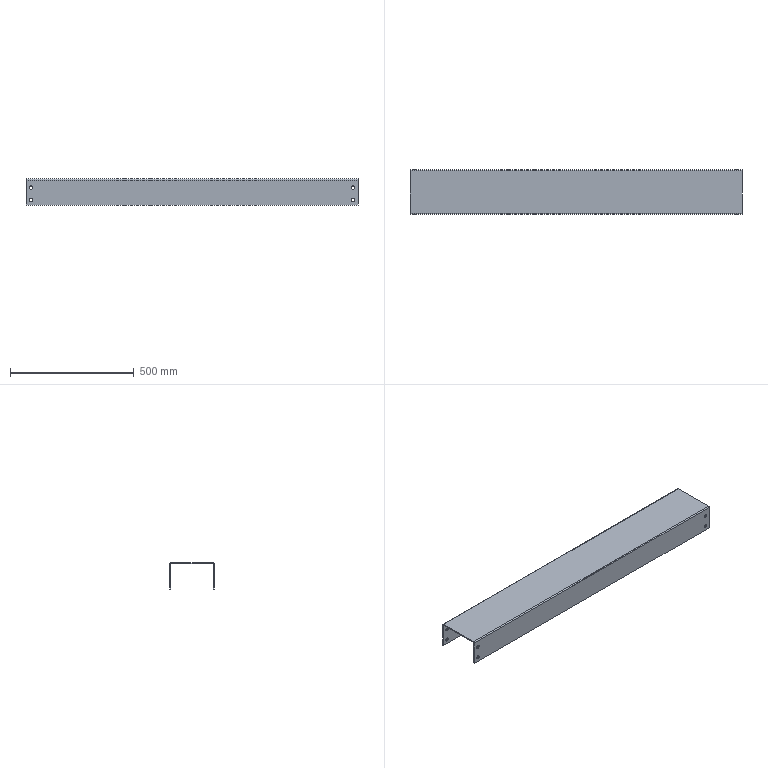Part | 1 solid | 38 faces | box 1340 x 180 x 105 mm | volume 2032472 mm3 | cylinder 20 | plane 18 | commonest cylinder face diameters 14 x16 0.4 x2 8.4 x2
STEP:
#1=CARTESIAN_POINT('',(650.,-90.,-92.));
#2=VERTEX_POINT('',#1);
#3=CARTESIAN_POINT('',(650.,-90.,-78.));
#4=VERTEX_POINT('',#3);
#5=CARTESIAN_POINT('',(650.,-90.,-85.));
#6=DIRECTION('',(0.,1.,0.));
#7=DIRECTION('',(0.,0.,1.));
#8=AXIS2_PLACEMENT_3D('',#5,#6,#7);
#9=CIRCLE('',#8,7.);
#10=EDGE_CURVE('',#2,#4,#9,.T.);
#11=ORIENTED_EDGE('',*,*,#10,.F.);
#12=CARTESIAN_POINT('',(650.,-86.,-92.));
#13=VERTEX_POINT('',#12);
#14=CARTESIAN_POINT('',(650.,-324.,-92.));
#15=DIRECTION('',(0.,1.,0.));
#16=VECTOR('',#15,1000.);
#17=LINE('',#14,#16);
#18=EDGE_CURVE('',#2,#13,#17,.T.);
#19=ORIENTED_EDGE('',*,*,#18,.T.);
#20=CARTESIAN_POINT('',(650.,-86.,-78.));
#21=VERTEX_POINT('',#20);
#22=CARTESIAN_POINT('',(650.,-86.,-85.));
#23=DIRECTION('',(0.,1.,0.));
#24=DIRECTION('',(0.,0.,1.));
#25=AXIS2_PLACEMENT_3D('',#22,#23,#24);
#26=CIRCLE('',#25,7.);
#27=EDGE_CURVE('',#13,#21,#26,.T.);
#28=ORIENTED_EDGE('',*,*,#27,.T.);
#29=CARTESIAN_POINT('',(650.,-324.,-78.));
#30=DIRECTION('',(0.,1.,0.));
#31=VECTOR('',#30,1000.);
#32=LINE('',#29,#31);
#33=EDGE_CURVE('',#4,#21,#32,.T.);
#34=ORIENTED_EDGE('',*,*,#33,.F.);
#35=EDGE_LOOP('',(#11,#19,#28,#34));
#36=FACE_OUTER_BOUND('',#35,.T.);
#37=CARTESIAN_POINT('',(650.,-324.,-85.));
#38=DIRECTION('',(0.,1.,0.));
#39=DIRECTION('',(0.,0.,1.));
#40=AXIS2_PLACEMENT_3D('',#37,#38,#39);
#41=CYLINDRICAL_SURFACE('',#40,7.);
#42=ADVANCED_FACE('',(#36),#41,.F.);
#43=CARTESIAN_POINT('',(650.,-90.,-42.));
#44=VERTEX_POINT('',#43);
#45=CARTESIAN_POINT('',(650.,-90.,-28.));
#46=VERTEX_POINT('',#45);
#47=CARTESIAN_POINT('',(650.,-90.,-35.));
#48=DIRECTION('',(0.,1.,0.));
#49=DIRECTION('',(0.,0.,1.));
#50=AXIS2_PLACEMENT_3D('',#47,#48,#49);
#51=CIRCLE('',#50,7.);
#52=EDGE_CURVE('',#44,#46,#51,.T.);
#53=ORIENTED_EDGE('',*,*,#52,.F.);
#54=CARTESIAN_POINT('',(650.,-86.,-42.));
#55=VERTEX_POINT('',#54);
#56=CARTESIAN_POINT('',(650.,-324.,-42.));
#57=DIRECTION('',(0.,1.,0.));
#58=VECTOR('',#57,1000.);
#59=LINE('',#56,#58);
#60=EDGE_CURVE('',#44,#55,#59,.T.);
#61=ORIENTED_EDGE('',*,*,#60,.T.);
#62=CARTESIAN_POINT('',(650.,-86.,-28.));
#63=VERTEX_POINT('',#62);
#64=CARTESIAN_POINT('',(650.,-86.,-35.));
#65=DIRECTION('',(0.,1.,0.));
#66=DIRECTION('',(0.,0.,1.));
#67=AXIS2_PLACEMENT_3D('',#64,#65,#66);
#68=CIRCLE('',#67,7.);
#69=EDGE_CURVE('',#55,#63,#68,.T.);
#70=ORIENTED_EDGE('',*,*,#69,.T.);
#71=CARTESIAN_POINT('',(650.,-324.,-28.));
#72=DIRECTION('',(0.,1.,0.));
#73=VECTOR('',#72,1000.);
#74=LINE('',#71,#73);
#75=EDGE_CURVE('',#46,#63,#74,.T.);
#76=ORIENTED_EDGE('',*,*,#75,.F.);
#77=EDGE_LOOP('',(#53,#61,#70,#76));
#78=FACE_OUTER_BOUND('',#77,.T.);
#79=CARTESIAN_POINT('',(650.,-324.,-35.));
#80=DIRECTION('',(0.,1.,0.));
#81=DIRECTION('',(0.,0.,1.));
#82=AXIS2_PLACEMENT_3D('',#79,#80,#81);
#83=CYLINDRICAL_SURFACE('',#82,7.);
#84=ADVANCED_FACE('',(#78),#83,.F.);
#85=CARTESIAN_POINT('',(-650.,-90.,-42.));
#86=VERTEX_POINT('',#85);
#87=CARTESIAN_POINT('',(-650.,-90.,-28.));
#88=VERTEX_POINT('',#87);
#89=CARTESIAN_POINT('',(-650.,-90.,-35.));
#90=DIRECTION('',(0.,1.,0.));
#91=DIRECTION('',(0.,0.,1.));
#92=AXIS2_PLACEMENT_3D('',#89,#90,#91);
#93=CIRCLE('',#92,7.);
#94=EDGE_CURVE('',#86,#88,#93,.T.);
#95=ORIENTED_EDGE('',*,*,#94,.F.);
#96=CARTESIAN_POINT('',(-650.,-86.,-42.));
#97=VERTEX_POINT('',#96);
#98=CARTESIAN_POINT('',(-650.,-324.,-42.));
#99=DIRECTION('',(0.,1.,0.));
#100=VECTOR('',#99,1000.);
#101=LINE('',#98,#100);
#102=EDGE_CURVE('',#86,#97,#101,.T.);
#103=ORIENTED_EDGE('',*,*,#102,.T.);
#104=CARTESIAN_POINT('',(-650.,-86.,-28.));
#105=VERTEX_POINT('',#104);
#106=CARTESIAN_POINT('',(-650.,-86.,-35.));
#107=DIRECTION('',(0.,1.,0.));
#108=DIRECTION('',(0.,0.,1.));
#109=AXIS2_PLACEMENT_3D('',#106,#107,#108);
#110=CIRCLE('',#109,7.);
#111=EDGE_CURVE('',#97,#105,#110,.T.);
#112=ORIENTED_EDGE('',*,*,#111,.T.);
#113=CARTESIAN_POINT('',(-650.,-324.,-28.));
#114=DIRECTION('',(0.,1.,0.));
#115=VECTOR('',#114,1000.);
#116=LINE('',#113,#115);
#117=EDGE_CURVE('',#88,#105,#116,.T.);
#118=ORIENTED_EDGE('',*,*,#117,.F.);
#119=EDGE_LOOP('',(#95,#103,#112,#118));
#120=FACE_OUTER_BOUND('',#119,.T.);
#121=CARTESIAN_POINT('',(-650.,-324.,-35.));
#122=DIRECTION('',(0.,1.,0.));
#123=DIRECTION('',(0.,0.,1.));
#124=AXIS2_PLACEMENT_3D('',#121,#122,#123);
#125=CYLINDRICAL_SURFACE('',#124,7.);
#126=ADVANCED_FACE('',(#120),#125,.F.);
#127=CARTESIAN_POINT('',(-650.,-90.,-92.));
#128=VERTEX_POINT('',#127);
#129=CARTESIAN_POINT('',(-650.,-90.,-78.));
#130=VERTEX_POINT('',#129);
#131=CARTESIAN_POINT('',(-650.,-90.,-85.));
#132=DIRECTION('',(0.,1.,0.));
#133=DIRECTION('',(0.,0.,1.));
#134=AXIS2_PLACEMENT_3D('',#131,#132,#133);
#135=CIRCLE('',#134,7.);
#136=EDGE_CURVE('',#128,#130,#135,.T.);
#137=ORIENTED_EDGE('',*,*,#136,.F.);
#138=CARTESIAN_POINT('',(-650.,-86.,-92.));
#139=VERTEX_POINT('',#138);
#140=CARTESIAN_POINT('',(-650.,-324.,-92.));
#141=DIRECTION('',(0.,1.,0.));
#142=VECTOR('',#141,1000.);
#143=LINE('',#140,#142);
#144=EDGE_CURVE('',#128,#139,#143,.T.);
#145=ORIENTED_EDGE('',*,*,#144,.T.);
#146=CARTESIAN_POINT('',(-650.,-86.,-78.));
#147=VERTEX_POINT('',#146);
#148=CARTESIAN_POINT('',(-650.,-86.,-85.));
#149=DIRECTION('',(0.,1.,0.));
#150=DIRECTION('',(0.,0.,1.));
#151=AXIS2_PLACEMENT_3D('',#148,#149,#150);
#152=CIRCLE('',#151,7.);
#153=EDGE_CURVE('',#139,#147,#152,.T.);
#154=ORIENTED_EDGE('',*,*,#153,.T.);
#155=CARTESIAN_POINT('',(-650.,-324.,-78.));
#156=DIRECTION('',(0.,1.,0.));
#157=VECTOR('',#156,1000.);
#158=LINE('',#155,#157);
#159=EDGE_CURVE('',#130,#147,#158,.T.);
#160=ORIENTED_EDGE('',*,*,#159,.F.);
#161=EDGE_LOOP('',(#137,#145,#154,#160));
#162=FACE_OUTER_BOUND('',#161,.T.);
#163=CARTESIAN_POINT('',(-650.,-324.,-85.));
#164=DIRECTION('',(0.,1.,0.));
#165=DIRECTION('',(0.,0.,1.));
#166=AXIS2_PLACEMENT_3D('',#163,#164,#165);
#167=CYLINDRICAL_SURFACE('',#166,7.);
#168=ADVANCED_FACE('',(#162),#167,.F.);
#169=CARTESIAN_POINT('',(650.,86.,-78.));
#170=VERTEX_POINT('',#169);
#171=CARTESIAN_POINT('',(650.,86.,-92.));
#172=VERTEX_POINT('',#171);
#173=CARTESIAN_POINT('',(650.,86.,-85.));
#174=DIRECTION('',(0.,-1.,0.));
#175=DIRECTION('',(0.,0.,-1.));
#176=AXIS2_PLACEMENT_3D('',#173,#174,#175);
#177=CIRCLE('',#176,7.);
#178=EDGE_CURVE('',#170,#172,#177,.T.);
#179=ORIENTED_EDGE('',*,*,#178,.T.);
#180=CARTESIAN_POINT('',(650.,90.,-92.));
#181=VERTEX_POINT('',#180);
#182=CARTESIAN_POINT('',(650.,-324.,-92.));
#183=DIRECTION('',(0.,1.,0.));
#184=VECTOR('',#183,1000.);
#185=LINE('',#182,#184);
#186=EDGE_CURVE('',#172,#181,#185,.T.);
#187=ORIENTED_EDGE('',*,*,#186,.T.);
#188=CARTESIAN_POINT('',(650.,90.,-78.));
#189=VERTEX_POINT('',#188);
#190=CARTESIAN_POINT('',(650.,90.,-85.));
#191=DIRECTION('',(0.,1.,0.));
#192=DIRECTION('',(0.,0.,-1.));
#193=AXIS2_PLACEMENT_3D('',#190,#191,#192);
#194=CIRCLE('',#193,7.);
#195=EDGE_CURVE('',#181,#189,#194,.T.);
#196=ORIENTED_EDGE('',*,*,#195,.T.);
#197=CARTESIAN_POINT('',(650.,-324.,-78.));
#198=DIRECTION('',(0.,1.,0.));
#199=VECTOR('',#198,1000.);
#200=LINE('',#197,#199);
#201=EDGE_CURVE('',#170,#189,#200,.T.);
#202=ORIENTED_EDGE('',*,*,#201,.F.);
#203=EDGE_LOOP('',(#179,#187,#196,#202));
#204=FACE_OUTER_BOUND('',#203,.T.);
#205=CARTESIAN_POINT('',(650.,-324.,-85.));
#206=DIRECTION('',(0.,1.,0.));
#207=DIRECTION('',(0.,0.,1.));
#208=AXIS2_PLACEMENT_3D('',#205,#206,#207);
#209=CYLINDRICAL_SURFACE('',#208,7.);
#210=ADVANCED_FACE('',(#204),#209,.F.);
#211=CARTESIAN_POINT('',(650.,86.,-28.));
#212=VERTEX_POINT('',#211);
#213=CARTESIAN_POINT('',(650.,86.,-42.));
#214=VERTEX_POINT('',#213);
#215=CARTESIAN_POINT('',(650.,86.,-35.));
#216=DIRECTION('',(0.,-1.,0.));
#217=DIRECTION('',(0.,0.,-1.));
#218=AXIS2_PLACEMENT_3D('',#215,#216,#217);
#219=CIRCLE('',#218,7.);
#220=EDGE_CURVE('',#212,#214,#219,.T.);
#221=ORIENTED_EDGE('',*,*,#220,.T.);
#222=CARTESIAN_POINT('',(650.,90.,-42.));
#223=VERTEX_POINT('',#222);
#224=CARTESIAN_POINT('',(650.,-324.,-42.));
#225=DIRECTION('',(0.,1.,0.));
#226=VECTOR('',#225,1000.);
#227=LINE('',#224,#226);
#228=EDGE_CURVE('',#214,#223,#227,.T.);
#229=ORIENTED_EDGE('',*,*,#228,.T.);
#230=CARTESIAN_POINT('',(650.,90.,-28.));
#231=VERTEX_POINT('',#230);
#232=CARTESIAN_POINT('',(650.,90.,-35.));
#233=DIRECTION('',(0.,1.,0.));
#234=DIRECTION('',(0.,0.,-1.));
#235=AXIS2_PLACEMENT_3D('',#232,#233,#234);
#236=CIRCLE('',#235,7.);
#237=EDGE_CURVE('',#223,#231,#236,.T.);
#238=ORIENTED_EDGE('',*,*,#237,.T.);
#239=CARTESIAN_POINT('',(650.,-324.,-28.));
#240=DIRECTION('',(0.,1.,0.));
#241=VECTOR('',#240,1000.);
#242=LINE('',#239,#241);
#243=EDGE_CURVE('',#212,#231,#242,.T.);
#244=ORIENTED_EDGE('',*,*,#243,.F.);
#245=EDGE_LOOP('',(#221,#229,#238,#244));
#246=FACE_OUTER_BOUND('',#245,.T.);
#247=CARTESIAN_POINT('',(650.,-324.,-35.));
#248=DIRECTION('',(0.,1.,0.));
#249=DIRECTION('',(0.,0.,1.));
#250=AXIS2_PLACEMENT_3D('',#247,#248,#249);
#251=CYLINDRICAL_SURFACE('',#250,7.);
#252=ADVANCED_FACE('',(#246),#251,.F.);
#253=CARTESIAN_POINT('',(-650.,86.,-28.));
#254=VERTEX_POINT('',#253);
#255=CARTESIAN_POINT('',(-650.,86.,-42.));
#256=VERTEX_POINT('',#255);
#257=CARTESIAN_POINT('',(-650.,86.,-35.));
#258=DIRECTION('',(0.,-1.,0.));
#259=DIRECTION('',(0.,0.,-1.));
#260=AXIS2_PLACEMENT_3D('',#257,#258,#259);
#261=CIRCLE('',#260,7.);
#262=EDGE_CURVE('',#254,#256,#261,.T.);
#263=ORIENTED_EDGE('',*,*,#262,.T.);
#264=CARTESIAN_POINT('',(-650.,90.,-42.));
#265=VERTEX_POINT('',#264);
#266=CARTESIAN_POINT('',(-650.,-324.,-42.));
#267=DIRECTION('',(0.,1.,0.));
#268=VECTOR('',#267,1000.);
#269=LINE('',#266,#268);
#270=EDGE_CURVE('',#256,#265,#269,.T.);
#271=ORIENTED_EDGE('',*,*,#270,.T.);
#272=CARTESIAN_POINT('',(-650.,90.,-28.));
#273=VERTEX_POINT('',#272);
#274=CARTESIAN_POINT('',(-650.,90.,-35.));
#275=DIRECTION('',(0.,1.,0.));
#276=DIRECTION('',(0.,0.,1.));
#277=AXIS2_PLACEMENT_3D('',#274,#275,#276);
#278=CIRCLE('',#277,7.);
#279=EDGE_CURVE('',#265,#273,#278,.T.);
#280=ORIENTED_EDGE('',*,*,#279,.T.);
#281=CARTESIAN_POINT('',(-650.,-324.,-28.));
#282=DIRECTION('',(0.,1.,0.));
#283=VECTOR('',#282,1000.);
#284=LINE('',#281,#283);
#285=EDGE_CURVE('',#254,#273,#284,.T.);
#286=ORIENTED_EDGE('',*,*,#285,.F.);
#287=EDGE_LOOP('',(#263,#271,#280,#286));
#288=FACE_OUTER_BOUND('',#287,.T.);
#289=CARTESIAN_POINT('',(-650.,-324.,-35.));
#290=DIRECTION('',(0.,1.,0.));
#291=DIRECTION('',(0.,0.,1.));
#292=AXIS2_PLACEMENT_3D('',#289,#290,#291);
#293=CYLINDRICAL_SURFACE('',#292,7.);
#294=ADVANCED_FACE('',(#288),#293,.F.);
#295=CARTESIAN_POINT('',(-650.,86.,-78.));
#296=VERTEX_POINT('',#295);
#297=CARTESIAN_POINT('',(-650.,86.,-92.));
#298=VERTEX_POINT('',#297);
#299=CARTESIAN_POINT('',(-650.,86.,-85.));
#300=DIRECTION('',(0.,-1.,0.));
#301=DIRECTION('',(0.,0.,-1.));
#302=AXIS2_PLACEMENT_3D('',#299,#300,#301);
#303=CIRCLE('',#302,7.);
#304=EDGE_CURVE('',#296,#298,#303,.T.);
#305=ORIENTED_EDGE('',*,*,#304,.T.);
#306=CARTESIAN_POINT('',(-650.,90.,-92.));
#307=VERTEX_POINT('',#306);
#308=CARTESIAN_POINT('',(-650.,-324.,-92.));
#309=DIRECTION('',(0.,1.,0.));
#310=VECTOR('',#309,1000.);
#311=LINE('',#308,#310);
#312=EDGE_CURVE('',#298,#307,#311,.T.);
#313=ORIENTED_EDGE('',*,*,#312,.T.);
#314=CARTESIAN_POINT('',(-650.,90.,-78.));
#315=VERTEX_POINT('',#314);
#316=CARTESIAN_POINT('',(-650.,90.,-85.));
#317=DIRECTION('',(0.,1.,0.));
#318=DIRECTION('',(0.,0.,1.));
#319=AXIS2_PLACEMENT_3D('',#316,#317,#318);
#320=CIRCLE('',#319,7.);
#321=EDGE_CURVE('',#307,#315,#320,.T.);
#322=ORIENTED_EDGE('',*,*,#321,.T.);
#323=CARTESIAN_POINT('',(-650.,-324.,-78.));
#324=DIRECTION('',(0.,1.,0.));
#325=VECTOR('',#324,1000.);
#326=LINE('',#323,#325);
#327=EDGE_CURVE('',#296,#315,#326,.T.);
#328=ORIENTED_EDGE('',*,*,#327,.F.);
#329=EDGE_LOOP('',(#305,#313,#322,#328));
#330=FACE_OUTER_BOUND('',#329,.T.);
#331=CARTESIAN_POINT('',(-650.,-324.,-85.));
#332=DIRECTION('',(0.,1.,0.));
#333=DIRECTION('',(0.,0.,1.));
#334=AXIS2_PLACEMENT_3D('',#331,#332,#333);
#335=CYLINDRICAL_SURFACE('',#334,7.);
#336=ADVANCED_FACE('',(#330),#335,.F.);
#337=CARTESIAN_POINT('',(670.,90.,-4.2));
#338=VERTEX_POINT('',#337);
#339=CARTESIAN_POINT('',(670.,86.,-4.2));
#340=VERTEX_POINT('',#339);
#341=CARTESIAN_POINT('',(670.,90.,-4.2));
#342=DIRECTION('',(0.,-1.,0.));
#343=VECTOR('',#342,1000.);
#344=LINE('',#341,#343);
#345=EDGE_CURVE('',#338,#340,#344,.T.);
#346=ORIENTED_EDGE('',*,*,#345,.F.);
#347=CARTESIAN_POINT('',(670.,85.8,0.));
#348=VERTEX_POINT('',#347);
#349=CARTESIAN_POINT('',(670.,85.8,-4.2));
#350=DIRECTION('',(1.,0.,0.));
#351=DIRECTION('',(0.,0.,1.));
#352=AXIS2_PLACEMENT_3D('',#349,#350,#351);
#353=CIRCLE('',#352,4.2);
#354=EDGE_CURVE('',#338,#348,#353,.T.);
#355=ORIENTED_EDGE('',*,*,#354,.T.);
#356=CARTESIAN_POINT('',(670.,85.8,-4.));
#357=VERTEX_POINT('',#356);
#358=CARTESIAN_POINT('',(670.,85.8,-4.));
#359=DIRECTION('',(0.,0.,1.));
#360=VECTOR('',#359,1000.);
#361=LINE('',#358,#360);
#362=EDGE_CURVE('',#357,#348,#361,.T.);
#363=ORIENTED_EDGE('',*,*,#362,.F.);
#364=CARTESIAN_POINT('',(670.,85.8,-4.2));
#365=DIRECTION('',(1.,0.,0.));
#366=DIRECTION('',(0.,0.,-1.));
#367=AXIS2_PLACEMENT_3D('',#364,#365,#366);
#368=CIRCLE('',#367,0.2);
#369=EDGE_CURVE('',#340,#357,#368,.T.);
#370=ORIENTED_EDGE('',*,*,#369,.F.);
#371=EDGE_LOOP('',(#346,#355,#363,#370));
#372=FACE_OUTER_BOUND('',#371,.T.);
#373=CARTESIAN_POINT('',(670.,90.,-4.2));
#374=DIRECTION('',(1.,0.,0.));
#375=DIRECTION('',(0.,0.,-1.));
#376=AXIS2_PLACEMENT_3D('',#373,#374,#375);
#377=PLANE('',#376);
#378=ADVANCED_FACE('',(#372),#377,.T.);
#379=CARTESIAN_POINT('',(670.,90.,-105.));
#380=VERTEX_POINT('',#379);
#381=CARTESIAN_POINT('',(670.,90.,-105.));
#382=DIRECTION('',(0.,0.,1.));
#383=VECTOR('',#382,1000.);
#384=LINE('',#381,#383);
#385=EDGE_CURVE('',#380,#338,#384,.T.);
#386=ORIENTED_EDGE('',*,*,#385,.T.);
#387=ORIENTED_EDGE('',*,*,#345,.T.);
#388=CARTESIAN_POINT('',(670.,86.,-105.));
#389=VERTEX_POINT('',#388);
#390=CARTESIAN_POINT('',(670.,86.,-105.));
#391=DIRECTION('',(0.,0.,1.));
#392=VECTOR('',#391,1000.);
#393=LINE('',#390,#392);
#394=EDGE_CURVE('',#389,#340,#393,.T.);
#395=ORIENTED_EDGE('',*,*,#394,.F.);
#396=CARTESIAN_POINT('',(670.,90.,-105.));
#397=DIRECTION('',(0.,-1.,0.));
#398=VECTOR('',#397,1000.);
#399=LINE('',#396,#398);
#400=EDGE_CURVE('',#380,#389,#399,.T.);
#401=ORIENTED_EDGE('',*,*,#400,.F.);
#402=EDGE_LOOP('',(#386,#387,#395,#401));
#403=FACE_OUTER_BOUND('',#402,.T.);
#404=CARTESIAN_POINT('',(670.,85.8,-4.));
#405=DIRECTION('',(1.,0.,0.));
#406=DIRECTION('',(0.,0.,-1.));
#407=AXIS2_PLACEMENT_3D('',#404,#405,#406);
#408=PLANE('',#407);
#409=ADVANCED_FACE('',(#403),#408,.T.);
#410=CARTESIAN_POINT('',(-670.,85.8,0.));
#411=VERTEX_POINT('',#410);
#412=CARTESIAN_POINT('',(-670.,85.8,-4.));
#413=VERTEX_POINT('',#412);
#414=CARTESIAN_POINT('',(-670.,85.8,0.));
#415=DIRECTION('',(0.,0.,-1.));
#416=VECTOR('',#415,1000.);
#417=LINE('',#414,#416);
#418=EDGE_CURVE('',#411,#413,#417,.T.);
#419=ORIENTED_EDGE('',*,*,#418,.F.);
#420=CARTESIAN_POINT('',(-670.,90.,-4.2));
#421=VERTEX_POINT('',#420);
#422=CARTESIAN_POINT('',(-670.,85.8,-4.2));
#423=DIRECTION('',(1.,0.,0.));
#424=DIRECTION('',(0.,0.,1.));
#425=AXIS2_PLACEMENT_3D('',#422,#423,#424);
#426=CIRCLE('',#425,4.2);
#427=EDGE_CURVE('',#421,#411,#426,.T.);
#428=ORIENTED_EDGE('',*,*,#427,.F.);
#429=CARTESIAN_POINT('',(-670.,86.,-4.2));
#430=VERTEX_POINT('',#429);
#431=CARTESIAN_POINT('',(-670.,86.,-4.2));
#432=DIRECTION('',(0.,1.,0.));
#433=VECTOR('',#432,1000.);
#434=LINE('',#431,#433);
#435=EDGE_CURVE('',#430,#421,#434,.T.);
#436=ORIENTED_EDGE('',*,*,#435,.F.);
#437=CARTESIAN_POINT('',(-670.,85.8,-4.2));
#438=DIRECTION('',(1.,0.,0.));
#439=DIRECTION('',(0.,0.,-1.));
#440=AXIS2_PLACEMENT_3D('',#437,#438,#439);
#441=CIRCLE('',#440,0.2);
#442=EDGE_CURVE('',#430,#413,#441,.T.);
#443=ORIENTED_EDGE('',*,*,#442,.T.);
#444=EDGE_LOOP('',(#419,#428,#436,#443));
#445=FACE_OUTER_BOUND('',#444,.T.);
#446=CARTESIAN_POINT('',(-670.,85.8,0.));
#447=DIRECTION('',(-1.,0.,0.));
#448=DIRECTION('',(0.,0.,1.));
#449=AXIS2_PLACEMENT_3D('',#446,#447,#448);
#450=PLANE('',#449);
#451=ADVANCED_FACE('',(#445),#450,.T.);
#452=CARTESIAN_POINT('',(-670.,-85.8,0.));
#453=VERTEX_POINT('',#452);
#454=CARTESIAN_POINT('',(-670.,90.,0.));
#455=DIRECTION('',(0.,-1.,0.));
#456=VECTOR('',#455,1000.);
#457=LINE('',#454,#456);
#458=EDGE_CURVE('',#411,#453,#457,.T.);
#459=ORIENTED_EDGE('',*,*,#458,.F.);
#460=ORIENTED_EDGE('',*,*,#418,.T.);
#461=CARTESIAN_POINT('',(-670.,-85.8,-4.));
#462=VERTEX_POINT('',#461);
#463=CARTESIAN_POINT('',(-670.,90.,-4.));
#464=DIRECTION('',(0.,-1.,0.));
#465=VECTOR('',#464,1000.);
#466=LINE('',#463,#465);
#467=EDGE_CURVE('',#413,#462,#466,.T.);
#468=ORIENTED_EDGE('',*,*,#467,.T.);
#469=CARTESIAN_POINT('',(-670.,-85.8,-4.));
#470=DIRECTION('',(0.,0.,1.));
#471=VECTOR('',#470,1000.);
#472=LINE('',#469,#471);
#473=EDGE_CURVE('',#462,#453,#472,.T.);
#474=ORIENTED_EDGE('',*,*,#473,.T.);
#475=EDGE_LOOP('',(#459,#460,#468,#474));
#476=FACE_OUTER_BOUND('',#475,.T.);
#477=CARTESIAN_POINT('',(-670.,86.,-4.2));
#478=DIRECTION('',(-1.,0.,0.));
#479=DIRECTION('',(0.,0.,1.));
#480=AXIS2_PLACEMENT_3D('',#477,#478,#479);
#481=PLANE('',#480);
#482=ADVANCED_FACE('',(#476),#481,.T.);
#483=CARTESIAN_POINT('',(670.,-85.8,0.));
#484=VERTEX_POINT('',#483);
#485=CARTESIAN_POINT('',(670.,-85.8,-4.));
#486=VERTEX_POINT('',#485);
#487=CARTESIAN_POINT('',(670.,-85.8,0.));
#488=DIRECTION('',(0.,0.,-1.));
#489=VECTOR('',#488,1000.);
#490=LINE('',#487,#489);
#491=EDGE_CURVE('',#484,#486,#490,.T.);
#492=ORIENTED_EDGE('',*,*,#491,.F.);
#493=CARTESIAN_POINT('',(670.,-90.,-4.2));
#494=VERTEX_POINT('',#493);
#495=CARTESIAN_POINT('',(670.,-85.8,-4.2));
#496=DIRECTION('',(1.,0.,0.));
#497=DIRECTION('',(0.,0.,1.));
#498=AXIS2_PLACEMENT_3D('',#495,#496,#497);
#499=CIRCLE('',#498,4.2);
#500=EDGE_CURVE('',#484,#494,#499,.T.);
#501=ORIENTED_EDGE('',*,*,#500,.T.);
#502=CARTESIAN_POINT('',(670.,-86.,-4.2));
#503=VERTEX_POINT('',#502);
#504=CARTESIAN_POINT('',(670.,-86.,-4.2));
#505=DIRECTION('',(0.,-1.,0.));
#506=VECTOR('',#505,1000.);
#507=LINE('',#504,#506);
#508=EDGE_CURVE('',#503,#494,#507,.T.);
#509=ORIENTED_EDGE('',*,*,#508,.F.);
#510=CARTESIAN_POINT('',(670.,-85.8,-4.2));
#511=DIRECTION('',(1.,0.,0.));
#512=DIRECTION('',(0.,0.,-1.));
#513=AXIS2_PLACEMENT_3D('',#510,#511,#512);
#514=CIRCLE('',#513,0.2);
#515=EDGE_CURVE('',#486,#503,#514,.T.);
#516=ORIENTED_EDGE('',*,*,#515,.F.);
#517=EDGE_LOOP('',(#492,#501,#509,#516));
#518=FACE_OUTER_BOUND('',#517,.T.);
#519=CARTESIAN_POINT('',(670.,-85.8,0.));
#520=DIRECTION('',(1.,0.,0.));
#521=DIRECTION('',(0.,0.,-1.));
#522=AXIS2_PLACEMENT_3D('',#519,#520,#521);
#523=PLANE('',#522);
#524=ADVANCED_FACE('',(#518),#523,.T.);
#525=CARTESIAN_POINT('',(670.,90.,0.));
#526=DIRECTION('',(0.,-1.,0.));
#527=VECTOR('',#526,1000.);
#528=LINE('',#525,#527);
#529=EDGE_CURVE('',#348,#484,#528,.T.);
#530=ORIENTED_EDGE('',*,*,#529,.T.);
#531=ORIENTED_EDGE('',*,*,#491,.T.);
#532=CARTESIAN_POINT('',(670.,90.,-4.));
#533=DIRECTION('',(0.,-1.,0.));
#534=VECTOR('',#533,1000.);
#535=LINE('',#532,#534);
#536=EDGE_CURVE('',#357,#486,#535,.T.);
#537=ORIENTED_EDGE('',*,*,#536,.F.);
#538=ORIENTED_EDGE('',*,*,#362,.T.);
#539=EDGE_LOOP('',(#530,#531,#537,#538));
#540=FACE_OUTER_BOUND('',#539,.T.);
#541=CARTESIAN_POINT('',(670.,-86.,-4.2));
#542=DIRECTION('',(1.,0.,0.));
#543=DIRECTION('',(0.,0.,-1.));
#544=AXIS2_PLACEMENT_3D('',#541,#542,#543);
#545=PLANE('',#544);
#546=ADVANCED_FACE('',(#540),#545,.T.);
#547=CARTESIAN_POINT('',(-670.,-90.,-4.2));
#548=VERTEX_POINT('',#547);
#549=CARTESIAN_POINT('',(-670.,-86.,-4.2));
#550=VERTEX_POINT('',#549);
#551=CARTESIAN_POINT('',(-670.,-90.,-4.2));
#552=DIRECTION('',(0.,1.,0.));
#553=VECTOR('',#552,1000.);
#554=LINE('',#551,#553);
#555=EDGE_CURVE('',#548,#550,#554,.T.);
#556=ORIENTED_EDGE('',*,*,#555,.F.);
#557=CARTESIAN_POINT('',(-670.,-85.8,-4.2));
#558=DIRECTION('',(1.,0.,0.));
#559=DIRECTION('',(0.,0.,1.));
#560=AXIS2_PLACEMENT_3D('',#557,#558,#559);
#561=CIRCLE('',#560,4.2);
#562=EDGE_CURVE('',#453,#548,#561,.T.);
#563=ORIENTED_EDGE('',*,*,#562,.F.);
#564=ORIENTED_EDGE('',*,*,#473,.F.);
#565=CARTESIAN_POINT('',(-670.,-85.8,-4.2));
#566=DIRECTION('',(1.,0.,0.));
#567=DIRECTION('',(0.,0.,-1.));
#568=AXIS2_PLACEMENT_3D('',#565,#566,#567);
#569=CIRCLE('',#568,0.2);
#570=EDGE_CURVE('',#462,#550,#569,.T.);
#571=ORIENTED_EDGE('',*,*,#570,.T.);
#572=EDGE_LOOP('',(#556,#563,#564,#571));
#573=FACE_OUTER_BOUND('',#572,.T.);
#574=CARTESIAN_POINT('',(-670.,-90.,-4.2));
#575=DIRECTION('',(-1.,0.,0.));
#576=DIRECTION('',(0.,0.,1.));
#577=AXIS2_PLACEMENT_3D('',#574,#575,#576);
#578=PLANE('',#577);
#579=ADVANCED_FACE('',(#573),#578,.T.);
#580=CARTESIAN_POINT('',(-670.,-90.,-105.));
#581=VERTEX_POINT('',#580);
#582=CARTESIAN_POINT('',(-670.,-90.,0.));
#583=DIRECTION('',(0.,0.,-1.));
#584=VECTOR('',#583,1000.);
#585=LINE('',#582,#584);
#586=EDGE_CURVE('',#548,#581,#585,.T.);
#587=ORIENTED_EDGE('',*,*,#586,.F.);
#588=ORIENTED_EDGE('',*,*,#555,.T.);
#589=CARTESIAN_POINT('',(-670.,-86.,-105.));
#590=VERTEX_POINT('',#589);
#591=CARTESIAN_POINT('',(-670.,-86.,0.));
#592=DIRECTION('',(0.,0.,-1.));
#593=VECTOR('',#592,1000.);
#594=LINE('',#591,#593);
#595=EDGE_CURVE('',#550,#590,#594,.T.);
#596=ORIENTED_EDGE('',*,*,#595,.T.);
#597=CARTESIAN_POINT('',(-670.,-86.,-105.));
#598=DIRECTION('',(0.,-1.,0.));
#599=VECTOR('',#598,1000.);
#600=LINE('',#597,#599);
#601=EDGE_CURVE('',#590,#581,#600,.T.);
#602=ORIENTED_EDGE('',*,*,#601,.T.);
#603=EDGE_LOOP('',(#587,#588,#596,#602));
#604=FACE_OUTER_BOUND('',#603,.T.);
#605=CARTESIAN_POINT('',(-670.,-85.8,-4.));
#606=DIRECTION('',(-1.,0.,0.));
#607=DIRECTION('',(0.,0.,1.));
#608=AXIS2_PLACEMENT_3D('',#605,#606,#607);
#609=PLANE('',#608);
#610=ADVANCED_FACE('',(#604),#609,.T.);
#611=CARTESIAN_POINT('',(650.,-90.,-85.));
#612=DIRECTION('',(0.,1.,0.));
#613=DIRECTION('',(0.,0.,1.));
#614=AXIS2_PLACEMENT_3D('',#611,#612,#613);
#615=CIRCLE('',#614,7.);
#616=EDGE_CURVE('',#4,#2,#615,.T.);
#617=ORIENTED_EDGE('',*,*,#616,.T.);
#618=ORIENTED_EDGE('',*,*,#10,.T.);
#619=EDGE_LOOP('',(#617,#618));
#620=FACE_BOUND('',#619,.T.);
#621=CARTESIAN_POINT('',(650.,-90.,-35.));
#622=DIRECTION('',(0.,1.,0.));
#623=DIRECTION('',(0.,0.,1.));
#624=AXIS2_PLACEMENT_3D('',#621,#622,#623);
#625=CIRCLE('',#624,7.);
#626=EDGE_CURVE('',#46,#44,#625,.T.);
#627=ORIENTED_EDGE('',*,*,#626,.T.);
#628=ORIENTED_EDGE('',*,*,#52,.T.);
#629=EDGE_LOOP('',(#627,#628));
#630=FACE_BOUND('',#629,.T.);
#631=CARTESIAN_POINT('',(-650.,-90.,-35.));
#632=DIRECTION('',(0.,1.,0.));
#633=DIRECTION('',(0.,0.,1.));
#634=AXIS2_PLACEMENT_3D('',#631,#632,#633);
#635=CIRCLE('',#634,7.);
#636=EDGE_CURVE('',#88,#86,#635,.T.);
#637=ORIENTED_EDGE('',*,*,#636,.T.);
#638=ORIENTED_EDGE('',*,*,#94,.T.);
#639=EDGE_LOOP('',(#637,#638));
#640=FACE_BOUND('',#639,.T.);
#641=CARTESIAN_POINT('',(-650.,-90.,-85.));
#642=DIRECTION('',(0.,1.,0.));
#643=DIRECTION('',(0.,0.,1.));
#644=AXIS2_PLACEMENT_3D('',#641,#642,#643);
#645=CIRCLE('',#644,7.);
#646=EDGE_CURVE('',#130,#128,#645,.T.);
#647=ORIENTED_EDGE('',*,*,#646,.T.);
#648=ORIENTED_EDGE('',*,*,#136,.T.);
#649=EDGE_LOOP('',(#647,#648));
#650=FACE_BOUND('',#649,.T.);
#651=ORIENTED_EDGE('',*,*,#586,.T.);
#652=CARTESIAN_POINT('',(670.,-90.,-105.));
#653=VERTEX_POINT('',#652);
#654=CARTESIAN_POINT('',(670.,-90.,-105.));
#655=DIRECTION('',(-1.,0.,0.));
#656=VECTOR('',#655,1000.);
#657=LINE('',#654,#656);
#658=EDGE_CURVE('',#653,#581,#657,.T.);
#659=ORIENTED_EDGE('',*,*,#658,.F.);
#660=CARTESIAN_POINT('',(670.,-90.,0.));
#661=DIRECTION('',(0.,0.,-1.));
#662=VECTOR('',#661,1000.);
#663=LINE('',#660,#662);
#664=EDGE_CURVE('',#494,#653,#663,.T.);
#665=ORIENTED_EDGE('',*,*,#664,.F.);
#666=CARTESIAN_POINT('',(670.,-90.,-4.2));
#667=DIRECTION('',(-1.,0.,0.));
#668=VECTOR('',#667,1000.);
#669=LINE('',#666,#668);
#670=EDGE_CURVE('',#494,#548,#669,.T.);
#671=ORIENTED_EDGE('',*,*,#670,.T.);
#672=EDGE_LOOP('',(#651,#659,#665,#671));
#673=FACE_OUTER_BOUND('',#672,.T.);
#674=CARTESIAN_POINT('',(670.,-90.,0.));
#675=DIRECTION('',(0.,1.,0.));
#676=DIRECTION('',(0.,0.,1.));
#677=AXIS2_PLACEMENT_3D('',#674,#675,#676);
#678=PLANE('',#677);
#679=ADVANCED_FACE('',(#620,#630,#640,#650,#673),#678,.F.);
#680=ORIENTED_EDGE('',*,*,#601,.F.);
#681=CARTESIAN_POINT('',(670.,-86.,-105.));
#682=VERTEX_POINT('',#681);
#683=CARTESIAN_POINT('',(670.,-86.,-105.));
#684=DIRECTION('',(-1.,0.,0.));
#685=VECTOR('',#684,1000.);
#686=LINE('',#683,#685);
#687=EDGE_CURVE('',#682,#590,#686,.T.);
#688=ORIENTED_EDGE('',*,*,#687,.F.);
#689=CARTESIAN_POINT('',(670.,-86.,-105.));
#690=DIRECTION('',(0.,-1.,0.));
#691=VECTOR('',#690,1000.);
#692=LINE('',#689,#691);
#693=EDGE_CURVE('',#682,#653,#692,.T.);
#694=ORIENTED_EDGE('',*,*,#693,.T.);
#695=ORIENTED_EDGE('',*,*,#658,.T.);
#696=EDGE_LOOP('',(#680,#688,#694,#695));
#697=FACE_OUTER_BOUND('',#696,.T.);
#698=CARTESIAN_POINT('',(670.,-86.,-105.));
#699=DIRECTION('',(0.,0.,-1.));
#700=DIRECTION('',(0.,1.,0.));
#701=AXIS2_PLACEMENT_3D('',#698,#699,#700);
#702=PLANE('',#701);
#703=ADVANCED_FACE('',(#697),#702,.T.);
#704=CARTESIAN_POINT('',(650.,-86.,-85.));
#705=DIRECTION('',(0.,1.,0.));
#706=DIRECTION('',(0.,0.,1.));
#707=AXIS2_PLACEMENT_3D('',#704,#705,#706);
#708=CIRCLE('',#707,7.);
#709=EDGE_CURVE('',#21,#13,#708,.T.);
#710=ORIENTED_EDGE('',*,*,#709,.F.);
#711=ORIENTED_EDGE('',*,*,#27,.F.);
#712=EDGE_LOOP('',(#710,#711));
#713=FACE_BOUND('',#712,.T.);
#714=CARTESIAN_POINT('',(650.,-86.,-35.));
#715=DIRECTION('',(0.,1.,0.));
#716=DIRECTION('',(0.,0.,1.));
#717=AXIS2_PLACEMENT_3D('',#714,#715,#716);
#718=CIRCLE('',#717,7.);
#719=EDGE_CURVE('',#63,#55,#718,.T.);
#720=ORIENTED_EDGE('',*,*,#719,.F.);
#721=ORIENTED_EDGE('',*,*,#69,.F.);
#722=EDGE_LOOP('',(#720,#721));
#723=FACE_BOUND('',#722,.T.);
#724=CARTESIAN_POINT('',(-650.,-86.,-35.));
#725=DIRECTION('',(0.,1.,0.));
#726=DIRECTION('',(0.,0.,1.));
#727=AXIS2_PLACEMENT_3D('',#724,#725,#726);
#728=CIRCLE('',#727,7.);
#729=EDGE_CURVE('',#105,#97,#728,.T.);
#730=ORIENTED_EDGE('',*,*,#729,.F.);
#731=ORIENTED_EDGE('',*,*,#111,.F.);
#732=EDGE_LOOP('',(#730,#731));
#733=FACE_BOUND('',#732,.T.);
#734=CARTESIAN_POINT('',(-650.,-86.,-85.));
#735=DIRECTION('',(0.,1.,0.));
#736=DIRECTION('',(0.,0.,1.));
#737=AXIS2_PLACEMENT_3D('',#734,#735,#736);
#738=CIRCLE('',#737,7.);
#739=EDGE_CURVE('',#147,#139,#738,.T.);
#740=ORIENTED_EDGE('',*,*,#739,.F.);
#741=ORIENTED_EDGE('',*,*,#153,.F.);
#742=EDGE_LOOP('',(#740,#741));
#743=FACE_BOUND('',#742,.T.);
#744=ORIENTED_EDGE('',*,*,#595,.F.);
#745=CARTESIAN_POINT('',(670.,-86.,-4.2));
#746=DIRECTION('',(-1.,0.,0.));
#747=VECTOR('',#746,1000.);
#748=LINE('',#745,#747);
#749=EDGE_CURVE('',#503,#550,#748,.T.);
#750=ORIENTED_EDGE('',*,*,#749,.F.);
#751=CARTESIAN_POINT('',(670.,-86.,0.));
#752=DIRECTION('',(0.,0.,-1.));
#753=VECTOR('',#752,1000.);
#754=LINE('',#751,#753);
#755=EDGE_CURVE('',#503,#682,#754,.T.);
#756=ORIENTED_EDGE('',*,*,#755,.T.);
#757=ORIENTED_EDGE('',*,*,#687,.T.);
#758=EDGE_LOOP('',(#744,#750,#756,#757));
#759=FACE_OUTER_BOUND('',#758,.T.);
#760=CARTESIAN_POINT('',(670.,-86.,0.));
#761=DIRECTION('',(0.,1.,0.));
#762=DIRECTION('',(0.,0.,1.));
#763=AXIS2_PLACEMENT_3D('',#760,#761,#762);
#764=PLANE('',#763);
#765=ADVANCED_FACE('',(#713,#723,#733,#743,#759),#764,.T.);
#766=ORIENTED_EDGE('',*,*,#570,.F.);
#767=CARTESIAN_POINT('',(670.,-85.8,-4.));
#768=DIRECTION('',(-1.,0.,0.));
#769=VECTOR('',#768,1000.);
#770=LINE('',#767,#769);
#771=EDGE_CURVE('',#486,#462,#770,.T.);
#772=ORIENTED_EDGE('',*,*,#771,.F.);
#773=ORIENTED_EDGE('',*,*,#515,.T.);
#774=ORIENTED_EDGE('',*,*,#749,.T.);
#775=EDGE_LOOP('',(#766,#772,#773,#774));
#776=FACE_OUTER_BOUND('',#775,.T.);
#777=CARTESIAN_POINT('',(670.,-85.8,-4.2));
#778=DIRECTION('',(-1.,0.,0.));
#779=DIRECTION('',(0.,0.,1.));
#780=AXIS2_PLACEMENT_3D('',#777,#778,#779);
#781=CYLINDRICAL_SURFACE('',#780,0.2);
#782=ADVANCED_FACE('',(#776),#781,.F.);
#783=ORIENTED_EDGE('',*,*,#467,.F.);
#784=CARTESIAN_POINT('',(670.,85.8,-4.));
#785=DIRECTION('',(-1.,0.,0.));
#786=VECTOR('',#785,1000.);
#787=LINE('',#784,#786);
#788=EDGE_CURVE('',#357,#413,#787,.T.);
#789=ORIENTED_EDGE('',*,*,#788,.F.);
#790=ORIENTED_EDGE('',*,*,#536,.T.);
#791=ORIENTED_EDGE('',*,*,#771,.T.);
#792=EDGE_LOOP('',(#783,#789,#790,#791));
#793=FACE_OUTER_BOUND('',#792,.T.);
#794=CARTESIAN_POINT('',(670.,90.,-4.));
#795=DIRECTION('',(0.,0.,-1.));
#796=DIRECTION('',(0.,1.,0.));
#797=AXIS2_PLACEMENT_3D('',#794,#795,#796);
#798=PLANE('',#797);
#799=ADVANCED_FACE('',(#793),#798,.T.);
#800=ORIENTED_EDGE('',*,*,#442,.F.);
#801=CARTESIAN_POINT('',(670.,86.,-4.2));
#802=DIRECTION('',(-1.,0.,0.));
#803=VECTOR('',#802,1000.);
#804=LINE('',#801,#803);
#805=EDGE_CURVE('',#340,#430,#804,.T.);
#806=ORIENTED_EDGE('',*,*,#805,.F.);
#807=ORIENTED_EDGE('',*,*,#369,.T.);
#808=ORIENTED_EDGE('',*,*,#788,.T.);
#809=EDGE_LOOP('',(#800,#806,#807,#808));
#810=FACE_OUTER_BOUND('',#809,.T.);
#811=CARTESIAN_POINT('',(670.,85.8,-4.2));
#812=DIRECTION('',(-1.,0.,0.));
#813=DIRECTION('',(0.,0.,1.));
#814=AXIS2_PLACEMENT_3D('',#811,#812,#813);
#815=CYLINDRICAL_SURFACE('',#814,0.2);
#816=ADVANCED_FACE('',(#810),#815,.F.);
#817=ORIENTED_EDGE('',*,*,#178,.F.);
#818=CARTESIAN_POINT('',(650.,86.,-85.));
#819=DIRECTION('',(0.,-1.,0.));
#820=DIRECTION('',(0.,0.,-1.));
#821=AXIS2_PLACEMENT_3D('',#818,#819,#820);
#822=CIRCLE('',#821,7.);
#823=EDGE_CURVE('',#172,#170,#822,.T.);
#824=ORIENTED_EDGE('',*,*,#823,.F.);
#825=EDGE_LOOP('',(#817,#824));
#826=FACE_BOUND('',#825,.T.);
#827=ORIENTED_EDGE('',*,*,#220,.F.);
#828=CARTESIAN_POINT('',(650.,86.,-35.));
#829=DIRECTION('',(0.,-1.,0.));
#830=DIRECTION('',(0.,0.,-1.));
#831=AXIS2_PLACEMENT_3D('',#828,#829,#830);
#832=CIRCLE('',#831,7.);
#833=EDGE_CURVE('',#214,#212,#832,.T.);
#834=ORIENTED_EDGE('',*,*,#833,.F.);
#835=EDGE_LOOP('',(#827,#834));
#836=FACE_BOUND('',#835,.T.);
#837=ORIENTED_EDGE('',*,*,#262,.F.);
#838=CARTESIAN_POINT('',(-650.,86.,-35.));
#839=DIRECTION('',(0.,-1.,0.));
#840=DIRECTION('',(0.,0.,-1.));
#841=AXIS2_PLACEMENT_3D('',#838,#839,#840);
#842=CIRCLE('',#841,7.);
#843=EDGE_CURVE('',#256,#254,#842,.T.);
#844=ORIENTED_EDGE('',*,*,#843,.F.);
#845=EDGE_LOOP('',(#837,#844));
#846=FACE_BOUND('',#845,.T.);
#847=ORIENTED_EDGE('',*,*,#304,.F.);
#848=CARTESIAN_POINT('',(-650.,86.,-85.));
#849=DIRECTION('',(0.,-1.,0.));
#850=DIRECTION('',(0.,0.,-1.));
#851=AXIS2_PLACEMENT_3D('',#848,#849,#850);
#852=CIRCLE('',#851,7.);
#853=EDGE_CURVE('',#298,#296,#852,.T.);
#854=ORIENTED_EDGE('',*,*,#853,.F.);
#855=EDGE_LOOP('',(#847,#854));
#856=FACE_BOUND('',#855,.T.);
#857=CARTESIAN_POINT('',(-670.,86.,-105.));
#858=VERTEX_POINT('',#857);
#859=CARTESIAN_POINT('',(-670.,86.,-105.));
#860=DIRECTION('',(0.,0.,1.));
#861=VECTOR('',#860,1000.);
#862=LINE('',#859,#861);
#863=EDGE_CURVE('',#858,#430,#862,.T.);
#864=ORIENTED_EDGE('',*,*,#863,.F.);
#865=CARTESIAN_POINT('',(670.,86.,-105.));
#866=DIRECTION('',(-1.,0.,0.));
#867=VECTOR('',#866,1000.);
#868=LINE('',#865,#867);
#869=EDGE_CURVE('',#389,#858,#868,.T.);
#870=ORIENTED_EDGE('',*,*,#869,.F.);
#871=ORIENTED_EDGE('',*,*,#394,.T.);
#872=ORIENTED_EDGE('',*,*,#805,.T.);
#873=EDGE_LOOP('',(#864,#870,#871,#872));
#874=FACE_OUTER_BOUND('',#873,.T.);
#875=CARTESIAN_POINT('',(670.,86.,-105.));
#876=DIRECTION('',(0.,-1.,0.));
#877=DIRECTION('',(0.,0.,-1.));
#878=AXIS2_PLACEMENT_3D('',#875,#876,#877);
#879=PLANE('',#878);
#880=ADVANCED_FACE('',(#826,#836,#846,#856,#874),#879,.T.);
#881=CARTESIAN_POINT('',(-670.,90.,-105.));
#882=VERTEX_POINT('',#881);
#883=CARTESIAN_POINT('',(-670.,90.,-105.));
#884=DIRECTION('',(0.,-1.,0.));
#885=VECTOR('',#884,1000.);
#886=LINE('',#883,#885);
#887=EDGE_CURVE('',#882,#858,#886,.T.);
#888=ORIENTED_EDGE('',*,*,#887,.F.);
#889=CARTESIAN_POINT('',(670.,90.,-105.));
#890=DIRECTION('',(-1.,0.,0.));
#891=VECTOR('',#890,1000.);
#892=LINE('',#889,#891);
#893=EDGE_CURVE('',#380,#882,#892,.T.);
#894=ORIENTED_EDGE('',*,*,#893,.F.);
#895=ORIENTED_EDGE('',*,*,#400,.T.);
#896=ORIENTED_EDGE('',*,*,#869,.T.);
#897=EDGE_LOOP('',(#888,#894,#895,#896));
#898=FACE_OUTER_BOUND('',#897,.T.);
#899=CARTESIAN_POINT('',(670.,90.,-105.));
#900=DIRECTION('',(0.,0.,-1.));
#901=DIRECTION('',(-1.,0.,0.));
#902=AXIS2_PLACEMENT_3D('',#899,#900,#901);
#903=PLANE('',#902);
#904=ADVANCED_FACE('',(#898),#903,.T.);
#905=CARTESIAN_POINT('',(650.,90.,-85.));
#906=DIRECTION('',(0.,1.,0.));
#907=DIRECTION('',(0.,0.,-1.));
#908=AXIS2_PLACEMENT_3D('',#905,#906,#907);
#909=CIRCLE('',#908,7.);
#910=EDGE_CURVE('',#189,#181,#909,.T.);
#911=ORIENTED_EDGE('',*,*,#910,.F.);
#912=ORIENTED_EDGE('',*,*,#195,.F.);
#913=EDGE_LOOP('',(#911,#912));
#914=FACE_BOUND('',#913,.T.);
#915=CARTESIAN_POINT('',(650.,90.,-35.));
#916=DIRECTION('',(0.,1.,0.));
#917=DIRECTION('',(0.,0.,-1.));
#918=AXIS2_PLACEMENT_3D('',#915,#916,#917);
#919=CIRCLE('',#918,7.);
#920=EDGE_CURVE('',#231,#223,#919,.T.);
#921=ORIENTED_EDGE('',*,*,#920,.F.);
#922=ORIENTED_EDGE('',*,*,#237,.F.);
#923=EDGE_LOOP('',(#921,#922));
#924=FACE_BOUND('',#923,.T.);
#925=CARTESIAN_POINT('',(-650.,90.,-35.));
#926=DIRECTION('',(0.,1.,0.));
#927=DIRECTION('',(0.,0.,1.));
#928=AXIS2_PLACEMENT_3D('',#925,#926,#927);
#929=CIRCLE('',#928,7.);
#930=EDGE_CURVE('',#273,#265,#929,.T.);
#931=ORIENTED_EDGE('',*,*,#930,.F.);
#932=ORIENTED_EDGE('',*,*,#279,.F.);
#933=EDGE_LOOP('',(#931,#932));
#934=FACE_BOUND('',#933,.T.);
#935=CARTESIAN_POINT('',(-650.,90.,-85.));
#936=DIRECTION('',(0.,1.,0.));
#937=DIRECTION('',(0.,0.,1.));
#938=AXIS2_PLACEMENT_3D('',#935,#936,#937);
#939=CIRCLE('',#938,7.);
#940=EDGE_CURVE('',#315,#307,#939,.T.);
#941=ORIENTED_EDGE('',*,*,#940,.F.);
#942=ORIENTED_EDGE('',*,*,#321,.F.);
#943=EDGE_LOOP('',(#941,#942));
#944=FACE_BOUND('',#943,.T.);
#945=CARTESIAN_POINT('',(-670.,90.,-105.));
#946=DIRECTION('',(0.,0.,1.));
#947=VECTOR('',#946,1000.);
#948=LINE('',#945,#947);
#949=EDGE_CURVE('',#882,#421,#948,.T.);
#950=ORIENTED_EDGE('',*,*,#949,.T.);
#951=CARTESIAN_POINT('',(670.,90.,-4.2));
#952=DIRECTION('',(-1.,0.,0.));
#953=VECTOR('',#952,1000.);
#954=LINE('',#951,#953);
#955=EDGE_CURVE('',#338,#421,#954,.T.);
#956=ORIENTED_EDGE('',*,*,#955,.F.);
#957=ORIENTED_EDGE('',*,*,#385,.F.);
#958=ORIENTED_EDGE('',*,*,#893,.T.);
#959=EDGE_LOOP('',(#950,#956,#957,#958));
#960=FACE_OUTER_BOUND('',#959,.T.);
#961=CARTESIAN_POINT('',(670.,90.,-105.));
#962=DIRECTION('',(0.,-1.,0.));
#963=DIRECTION('',(0.,0.,-1.));
#964=AXIS2_PLACEMENT_3D('',#961,#962,#963);
#965=PLANE('',#964);
#966=ADVANCED_FACE('',(#914,#924,#934,#944,#960),#965,.F.);
#967=ORIENTED_EDGE('',*,*,#427,.T.);
#968=CARTESIAN_POINT('',(670.,85.8,0.));
#969=DIRECTION('',(-1.,0.,0.));
#970=VECTOR('',#969,1000.);
#971=LINE('',#968,#970);
#972=EDGE_CURVE('',#348,#411,#971,.T.);
#973=ORIENTED_EDGE('',*,*,#972,.F.);
#974=ORIENTED_EDGE('',*,*,#354,.F.);
#975=ORIENTED_EDGE('',*,*,#955,.T.);
#976=EDGE_LOOP('',(#967,#973,#974,#975));
#977=FACE_OUTER_BOUND('',#976,.T.);
#978=CARTESIAN_POINT('',(670.,85.8,-4.2));
#979=DIRECTION('',(-1.,0.,0.));
#980=DIRECTION('',(0.,0.,1.));
#981=AXIS2_PLACEMENT_3D('',#978,#979,#980);
#982=CYLINDRICAL_SURFACE('',#981,4.2);
#983=ADVANCED_FACE('',(#977),#982,.T.);
#984=ORIENTED_EDGE('',*,*,#458,.T.);
#985=CARTESIAN_POINT('',(670.,-85.8,0.));
#986=DIRECTION('',(-1.,0.,0.));
#987=VECTOR('',#986,1000.);
#988=LINE('',#985,#987);
#989=EDGE_CURVE('',#484,#453,#988,.T.);
#990=ORIENTED_EDGE('',*,*,#989,.F.);
#991=ORIENTED_EDGE('',*,*,#529,.F.);
#992=ORIENTED_EDGE('',*,*,#972,.T.);
#993=EDGE_LOOP('',(#984,#990,#991,#992));
#994=FACE_OUTER_BOUND('',#993,.T.);
#995=CARTESIAN_POINT('',(670.,90.,0.));
#996=DIRECTION('',(0.,0.,-1.));
#997=DIRECTION('',(0.,1.,0.));
#998=AXIS2_PLACEMENT_3D('',#995,#996,#997);
#999=PLANE('',#998);
#1000=ADVANCED_FACE('',(#994),#999,.F.);
#1001=ORIENTED_EDGE('',*,*,#562,.T.);
#1002=ORIENTED_EDGE('',*,*,#670,.F.);
#1003=ORIENTED_EDGE('',*,*,#500,.F.);
#1004=ORIENTED_EDGE('',*,*,#989,.T.);
#1005=EDGE_LOOP('',(#1001,#1002,#1003,#1004));
#1006=FACE_OUTER_BOUND('',#1005,.T.);
#1007=CARTESIAN_POINT('',(670.,-85.8,-4.2));
#1008=DIRECTION('',(-1.,0.,0.));
#1009=DIRECTION('',(0.,0.,1.));
#1010=AXIS2_PLACEMENT_3D('',#1007,#1008,#1009);
#1011=CYLINDRICAL_SURFACE('',#1010,4.2);
#1012=ADVANCED_FACE('',(#1006),#1011,.T.);
#1013=ORIENTED_EDGE('',*,*,#664,.T.);
#1014=ORIENTED_EDGE('',*,*,#693,.F.);
#1015=ORIENTED_EDGE('',*,*,#755,.F.);
#1016=ORIENTED_EDGE('',*,*,#508,.T.);
#1017=EDGE_LOOP('',(#1013,#1014,#1015,#1016));
#1018=FACE_OUTER_BOUND('',#1017,.T.);
#1019=CARTESIAN_POINT('',(670.,-85.8,-4.2));
#1020=DIRECTION('',(1.,0.,0.));
#1021=DIRECTION('',(0.,0.,-1.));
#1022=AXIS2_PLACEMENT_3D('',#1019,#1020,#1021);
#1023=PLANE('',#1022);
#1024=ADVANCED_FACE('',(#1018),#1023,.T.);
#1025=ORIENTED_EDGE('',*,*,#863,.T.);
#1026=ORIENTED_EDGE('',*,*,#435,.T.);
#1027=ORIENTED_EDGE('',*,*,#949,.F.);
#1028=ORIENTED_EDGE('',*,*,#887,.T.);
#1029=EDGE_LOOP('',(#1025,#1026,#1027,#1028));
#1030=FACE_OUTER_BOUND('',#1029,.T.);
#1031=CARTESIAN_POINT('',(-670.,-85.8,-4.2));
#1032=DIRECTION('',(1.,0.,0.));
#1033=DIRECTION('',(0.,0.,-1.));
#1034=AXIS2_PLACEMENT_3D('',#1031,#1032,#1033);
#1035=PLANE('',#1034);
#1036=ADVANCED_FACE('',(#1030),#1035,.F.);
#1037=ORIENTED_EDGE('',*,*,#312,.F.);
#1038=ORIENTED_EDGE('',*,*,#853,.T.);
#1039=ORIENTED_EDGE('',*,*,#327,.T.);
#1040=ORIENTED_EDGE('',*,*,#940,.T.);
#1041=EDGE_LOOP('',(#1037,#1038,#1039,#1040));
#1042=FACE_OUTER_BOUND('',#1041,.T.);
#1043=CARTESIAN_POINT('',(-650.,-324.,-85.));
#1044=DIRECTION('',(0.,1.,0.));
#1045=DIRECTION('',(0.,0.,1.));
#1046=AXIS2_PLACEMENT_3D('',#1043,#1044,#1045);
#1047=CYLINDRICAL_SURFACE('',#1046,7.);
#1048=ADVANCED_FACE('',(#1042),#1047,.F.);
#1049=ORIENTED_EDGE('',*,*,#270,.F.);
#1050=ORIENTED_EDGE('',*,*,#843,.T.);
#1051=ORIENTED_EDGE('',*,*,#285,.T.);
#1052=ORIENTED_EDGE('',*,*,#930,.T.);
#1053=EDGE_LOOP('',(#1049,#1050,#1051,#1052));
#1054=FACE_OUTER_BOUND('',#1053,.T.);
#1055=CARTESIAN_POINT('',(-650.,-324.,-35.));
#1056=DIRECTION('',(0.,1.,0.));
#1057=DIRECTION('',(0.,0.,1.));
#1058=AXIS2_PLACEMENT_3D('',#1055,#1056,#1057);
#1059=CYLINDRICAL_SURFACE('',#1058,7.);
#1060=ADVANCED_FACE('',(#1054),#1059,.F.);
#1061=ORIENTED_EDGE('',*,*,#228,.F.);
#1062=ORIENTED_EDGE('',*,*,#833,.T.);
#1063=ORIENTED_EDGE('',*,*,#243,.T.);
#1064=ORIENTED_EDGE('',*,*,#920,.T.);
#1065=EDGE_LOOP('',(#1061,#1062,#1063,#1064));
#1066=FACE_OUTER_BOUND('',#1065,.T.);
#1067=CARTESIAN_POINT('',(650.,-324.,-35.));
#1068=DIRECTION('',(0.,1.,0.));
#1069=DIRECTION('',(0.,0.,1.));
#1070=AXIS2_PLACEMENT_3D('',#1067,#1068,#1069);
#1071=CYLINDRICAL_SURFACE('',#1070,7.);
#1072=ADVANCED_FACE('',(#1066),#1071,.F.);
#1073=ORIENTED_EDGE('',*,*,#186,.F.);
#1074=ORIENTED_EDGE('',*,*,#823,.T.);
#1075=ORIENTED_EDGE('',*,*,#201,.T.);
#1076=ORIENTED_EDGE('',*,*,#910,.T.);
#1077=EDGE_LOOP('',(#1073,#1074,#1075,#1076));
#1078=FACE_OUTER_BOUND('',#1077,.T.);
#1079=CARTESIAN_POINT('',(650.,-324.,-85.));
#1080=DIRECTION('',(0.,1.,0.));
#1081=DIRECTION('',(0.,0.,1.));
#1082=AXIS2_PLACEMENT_3D('',#1079,#1080,#1081);
#1083=CYLINDRICAL_SURFACE('',#1082,7.);
#1084=ADVANCED_FACE('',(#1078),#1083,.F.);
#1085=ORIENTED_EDGE('',*,*,#144,.F.);
#1086=ORIENTED_EDGE('',*,*,#646,.F.);
#1087=ORIENTED_EDGE('',*,*,#159,.T.);
#1088=ORIENTED_EDGE('',*,*,#739,.T.);
#1089=EDGE_LOOP('',(#1085,#1086,#1087,#1088));
#1090=FACE_OUTER_BOUND('',#1089,.T.);
#1091=CARTESIAN_POINT('',(-650.,-324.,-85.));
#1092=DIRECTION('',(0.,1.,0.));
#1093=DIRECTION('',(0.,0.,1.));
#1094=AXIS2_PLACEMENT_3D('',#1091,#1092,#1093);
#1095=CYLINDRICAL_SURFACE('',#1094,7.);
#1096=ADVANCED_FACE('',(#1090),#1095,.F.);
#1097=ORIENTED_EDGE('',*,*,#102,.F.);
#1098=ORIENTED_EDGE('',*,*,#636,.F.);
#1099=ORIENTED_EDGE('',*,*,#117,.T.);
#1100=ORIENTED_EDGE('',*,*,#729,.T.);
#1101=EDGE_LOOP('',(#1097,#1098,#1099,#1100));
#1102=FACE_OUTER_BOUND('',#1101,.T.);
#1103=CARTESIAN_POINT('',(-650.,-324.,-35.));
#1104=DIRECTION('',(0.,1.,0.));
#1105=DIRECTION('',(0.,0.,1.));
#1106=AXIS2_PLACEMENT_3D('',#1103,#1104,#1105);
#1107=CYLINDRICAL_SURFACE('',#1106,7.);
#1108=ADVANCED_FACE('',(#1102),#1107,.F.);
#1109=ORIENTED_EDGE('',*,*,#60,.F.);
#1110=ORIENTED_EDGE('',*,*,#626,.F.);
#1111=ORIENTED_EDGE('',*,*,#75,.T.);
#1112=ORIENTED_EDGE('',*,*,#719,.T.);
#1113=EDGE_LOOP('',(#1109,#1110,#1111,#1112));
#1114=FACE_OUTER_BOUND('',#1113,.T.);
#1115=CARTESIAN_POINT('',(650.,-324.,-35.));
#1116=DIRECTION('',(0.,1.,0.));
#1117=DIRECTION('',(0.,0.,1.));
#1118=AXIS2_PLACEMENT_3D('',#1115,#1116,#1117);
#1119=CYLINDRICAL_SURFACE('',#1118,7.);
#1120=ADVANCED_FACE('',(#1114),#1119,.F.);
#1121=ORIENTED_EDGE('',*,*,#18,.F.);
#1122=ORIENTED_EDGE('',*,*,#616,.F.);
#1123=ORIENTED_EDGE('',*,*,#33,.T.);
#1124=ORIENTED_EDGE('',*,*,#709,.T.);
#1125=EDGE_LOOP('',(#1121,#1122,#1123,#1124));
#1126=FACE_OUTER_BOUND('',#1125,.T.);
#1127=CARTESIAN_POINT('',(650.,-324.,-85.));
#1128=DIRECTION('',(0.,1.,0.));
#1129=DIRECTION('',(0.,0.,1.));
#1130=AXIS2_PLACEMENT_3D('',#1127,#1128,#1129);
#1131=CYLINDRICAL_SURFACE('',#1130,7.);
#1132=ADVANCED_FACE('',(#1126),#1131,.F.);
#1133=CLOSED_SHELL('',(#42,#84,#126,#168,#210,#252,#294,#336,#378,#409,#451,#482,#524,#546,#579,#610,#679,#703,#765,#782,#799,#816,#880,#904,#966,#983,#1000,#1012,#1024,#1036,#1048,#1060,#1072,#1084,#1096,#1108,#1120,#1132));
#1134=MANIFOLD_SOLID_BREP('',#1133);
#1135=CARTESIAN_POINT('',(0.,0.,0.));
#1136=DIRECTION('',(0.,0.,1.));
#1137=DIRECTION('',(1.,0.,0.));
#1138=AXIS2_PLACEMENT_3D('',#1135,#1136,#1137);
#1139=(LENGTH_UNIT()NAMED_UNIT(*)SI_UNIT(.MILLI.,.METRE.));
#1140=UNCERTAINTY_MEASURE_WITH_UNIT(LENGTH_MEASURE(0.00001),#1139,'','');
#1141=(NAMED_UNIT(*)PLANE_ANGLE_UNIT()SI_UNIT($,.RADIAN.));
#1142=(NAMED_UNIT(*)SI_UNIT($,.STERADIAN.)SOLID_ANGLE_UNIT());
#1143=(GEOMETRIC_REPRESENTATION_CONTEXT(3)GLOBAL_UNCERTAINTY_ASSIGNED_CONTEXT((#1140))GLOBAL_UNIT_ASSIGNED_CONTEXT((#1139,#1141,#1142))REPRESENTATION_CONTEXT('',''));
#1144=ADVANCED_BREP_SHAPE_REPRESENTATION('',(#1134,#1138),#1143);